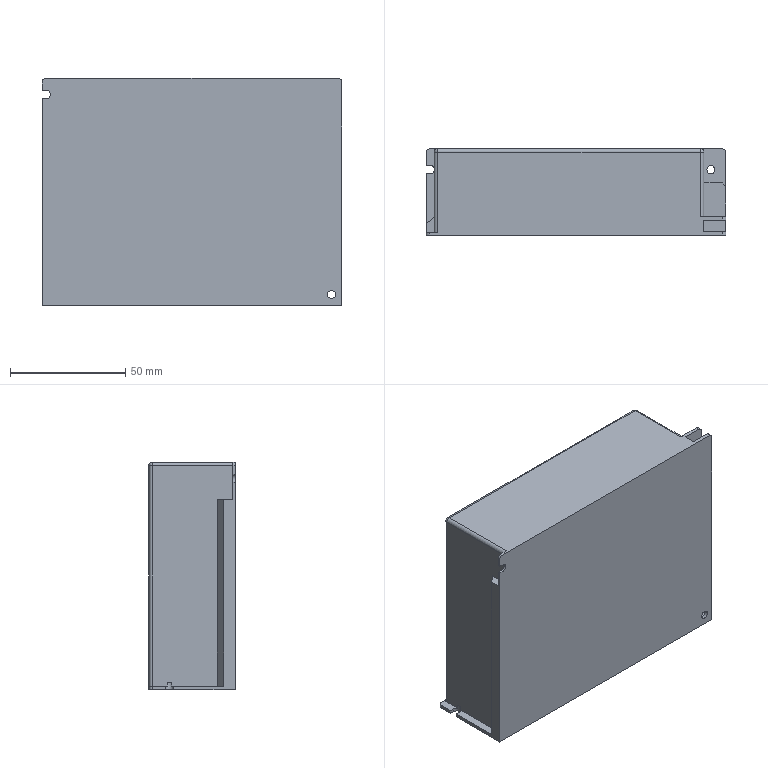Part | STEP file | Power supply 220-24 | 1 solid | 616 faces | box 130 x 37.5 x 98.5 mm | volume 426318 mm3 | cylinder 376 | plane 238 | sphere 2 | commonest cylinder face diameters 4.5 x360 3 x10 3.5 x6